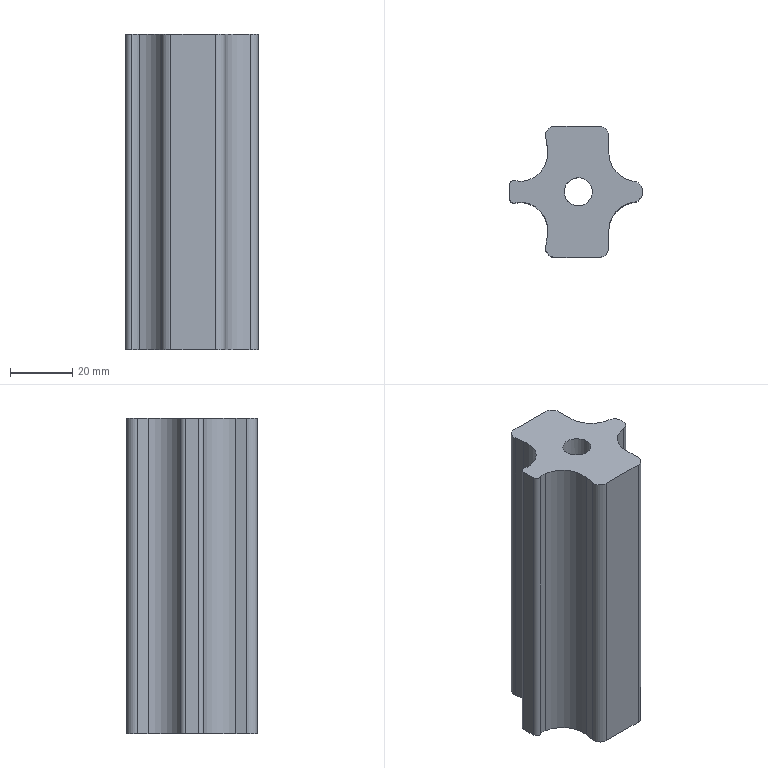Part | STEP file | PN_0031_id862_x_t | 1 solid | 27 faces | box 42.5 x 42 x 101 mm | volume 91343 mm3 | cylinder 16 | plane 11 | commonest cylinder face diameters 6 x6 18.5 x4 3 x2 10 x2 9 x1 14 x1
STEP:
#1=CARTESIAN_POINT('',(343.5,-0.3422,-6.));
#2=VERTEX_POINT('',#1);
#3=CARTESIAN_POINT('',(340.867,-3.32,-6.));
#4=VERTEX_POINT('',#3);
#5=CARTESIAN_POINT('',(340.5,-0.3422,-6.));
#6=DIRECTION('',(0.,0.,-1.));
#7=DIRECTION('',(1.,0.,0.));
#8=AXIS2_PLACEMENT_3D('',#5,#6,#7);
#9=CIRCLE('',#8,3.);
#10=EDGE_CURVE('',#2,#4,#9,.T.);
#11=ORIENTED_EDGE('',*,*,#10,.F.);
#12=CARTESIAN_POINT('',(343.5,-0.3422,95.));
#13=VERTEX_POINT('',#12);
#14=CARTESIAN_POINT('',(343.5,-0.3422,11.));
#15=DIRECTION('',(0.,0.,-1.));
#16=VECTOR('',#15,1.);
#17=LINE('',#14,#16);
#18=EDGE_CURVE('',#13,#2,#17,.T.);
#19=ORIENTED_EDGE('',*,*,#18,.F.);
#20=CARTESIAN_POINT('',(340.867,-3.32,95.));
#21=VERTEX_POINT('',#20);
#22=CARTESIAN_POINT('',(340.5,-0.3422,95.));
#23=DIRECTION('',(0.,0.,-1.));
#24=DIRECTION('',(-1.,0.,0.));
#25=AXIS2_PLACEMENT_3D('',#22,#23,#24);
#26=CIRCLE('',#25,3.);
#27=EDGE_CURVE('',#13,#21,#26,.T.);
#28=ORIENTED_EDGE('',*,*,#27,.T.);
#29=CARTESIAN_POINT('',(340.867,-3.32,11.));
#30=DIRECTION('',(0.,0.,-1.));
#31=VECTOR('',#30,1.);
#32=LINE('',#29,#31);
#33=EDGE_CURVE('',#21,#4,#32,.T.);
#34=ORIENTED_EDGE('',*,*,#33,.T.);
#35=EDGE_LOOP('',(#11,#19,#28,#34));
#36=FACE_OUTER_BOUND('',#35,.T.);
#37=CARTESIAN_POINT('',(340.5,-0.3422,11.));
#38=DIRECTION('',(0.,0.,-1.));
#39=DIRECTION('',(-1.,0.,0.));
#40=AXIS2_PLACEMENT_3D('',#37,#38,#39);
#41=CYLINDRICAL_SURFACE('',#40,3.);
#42=ADVANCED_FACE('',(#36),#41,.T.);
#43=ORIENTED_EDGE('',*,*,#33,.F.);
#44=CARTESIAN_POINT('',(332.75,-12.5,95.));
#45=VERTEX_POINT('',#44);
#46=CARTESIAN_POINT('',(342.,-12.5,95.));
#47=DIRECTION('',(0.,0.,1.));
#48=DIRECTION('',(-1.,0.,0.));
#49=AXIS2_PLACEMENT_3D('',#46,#47,#48);
#50=CIRCLE('',#49,9.25);
#51=EDGE_CURVE('',#21,#45,#50,.T.);
#52=ORIENTED_EDGE('',*,*,#51,.T.);
#53=CARTESIAN_POINT('',(332.75,-12.5,-6.));
#54=VERTEX_POINT('',#53);
#55=CARTESIAN_POINT('',(332.75,-12.5,11.));
#56=DIRECTION('',(0.,0.,-1.));
#57=VECTOR('',#56,1.);
#58=LINE('',#55,#57);
#59=EDGE_CURVE('',#45,#54,#58,.T.);
#60=ORIENTED_EDGE('',*,*,#59,.T.);
#61=CARTESIAN_POINT('',(342.,-12.5,-6.));
#62=DIRECTION('',(0.,0.,1.));
#63=DIRECTION('',(1.,0.,0.));
#64=AXIS2_PLACEMENT_3D('',#61,#62,#63);
#65=CIRCLE('',#64,9.25);
#66=EDGE_CURVE('',#4,#54,#65,.T.);
#67=ORIENTED_EDGE('',*,*,#66,.F.);
#68=EDGE_LOOP('',(#43,#52,#60,#67));
#69=FACE_OUTER_BOUND('',#68,.T.);
#70=CARTESIAN_POINT('',(342.,-12.5,11.));
#71=DIRECTION('',(0.,0.,-1.));
#72=DIRECTION('',(-1.,0.,0.));
#73=AXIS2_PLACEMENT_3D('',#70,#71,#72);
#74=CYLINDRICAL_SURFACE('',#73,9.25);
#75=ADVANCED_FACE('',(#69),#74,.F.);
#76=CARTESIAN_POINT('',(332.75,-18.,95.));
#77=VERTEX_POINT('',#76);
#78=CARTESIAN_POINT('',(332.75,24.687,95.));
#79=DIRECTION('',(0.,-1.,0.));
#80=VECTOR('',#79,1.);
#81=LINE('',#78,#80);
#82=EDGE_CURVE('',#45,#77,#81,.T.);
#83=ORIENTED_EDGE('',*,*,#82,.T.);
#84=CARTESIAN_POINT('',(332.75,-18.,-6.));
#85=VERTEX_POINT('',#84);
#86=CARTESIAN_POINT('',(332.75,-18.,11.));
#87=DIRECTION('',(0.,0.,-1.));
#88=VECTOR('',#87,1.);
#89=LINE('',#86,#88);
#90=EDGE_CURVE('',#77,#85,#89,.T.);
#91=ORIENTED_EDGE('',*,*,#90,.T.);
#92=CARTESIAN_POINT('',(332.75,-96.152,-6.));
#93=DIRECTION('',(0.,-1.,0.));
#94=VECTOR('',#93,1.);
#95=LINE('',#92,#94);
#96=EDGE_CURVE('',#54,#85,#95,.T.);
#97=ORIENTED_EDGE('',*,*,#96,.F.);
#98=ORIENTED_EDGE('',*,*,#59,.F.);
#99=EDGE_LOOP('',(#83,#91,#97,#98));
#100=FACE_OUTER_BOUND('',#99,.T.);
#101=CARTESIAN_POINT('',(332.75,-71.15,11.));
#102=DIRECTION('',(-1.,0.,0.));
#103=DIRECTION('',(0.,1.,0.));
#104=AXIS2_PLACEMENT_3D('',#101,#102,#103);
#105=PLANE('',#104);
#106=ADVANCED_FACE('',(#100),#105,.F.);
#107=CARTESIAN_POINT('',(329.75,-21.,-6.));
#108=VERTEX_POINT('',#107);
#109=CARTESIAN_POINT('',(315.473,-21.,-6.));
#110=VERTEX_POINT('',#109);
#111=CARTESIAN_POINT('',(-201.609,-21.,-6.));
#112=DIRECTION('',(-1.,0.,0.));
#113=VECTOR('',#112,1.);
#114=LINE('',#111,#113);
#115=EDGE_CURVE('',#108,#110,#114,.T.);
#116=ORIENTED_EDGE('',*,*,#115,.F.);
#117=CARTESIAN_POINT('',(329.75,-21.,95.));
#118=VERTEX_POINT('',#117);
#119=CARTESIAN_POINT('',(329.75,-21.,11.));
#120=DIRECTION('',(0.,0.,1.));
#121=VECTOR('',#120,1.);
#122=LINE('',#119,#121);
#123=EDGE_CURVE('',#108,#118,#122,.T.);
#124=ORIENTED_EDGE('',*,*,#123,.T.);
#125=CARTESIAN_POINT('',(315.473,-21.,95.));
#126=VERTEX_POINT('',#125);
#127=CARTESIAN_POINT('',(-114.973,-21.,95.));
#128=DIRECTION('',(-1.,0.,0.));
#129=VECTOR('',#128,1.);
#130=LINE('',#127,#129);
#131=EDGE_CURVE('',#118,#126,#130,.T.);
#132=ORIENTED_EDGE('',*,*,#131,.T.);
#133=CARTESIAN_POINT('',(315.473,-21.,11.));
#134=DIRECTION('',(0.,0.,-1.));
#135=VECTOR('',#134,1.);
#136=LINE('',#133,#135);
#137=EDGE_CURVE('',#126,#110,#136,.T.);
#138=ORIENTED_EDGE('',*,*,#137,.T.);
#139=EDGE_LOOP('',(#116,#124,#132,#138));
#140=FACE_OUTER_BOUND('',#139,.T.);
#141=CARTESIAN_POINT('',(546.19,-21.,11.));
#142=DIRECTION('',(0.,-1.,0.));
#143=DIRECTION('',(-1.,0.,0.));
#144=AXIS2_PLACEMENT_3D('',#141,#142,#143);
#145=PLANE('',#144);
#146=ADVANCED_FACE('',(#140),#145,.T.);
#147=CARTESIAN_POINT('',(312.518,-17.482,-6.));
#148=VERTEX_POINT('',#147);
#149=CARTESIAN_POINT('',(313.111,-14.097,-6.));
#150=VERTEX_POINT('',#149);
#151=CARTESIAN_POINT('',(283.807,-181.252,-6.));
#152=DIRECTION('',(0.1727,0.985,0.));
#153=VECTOR('',#152,1.);
#154=LINE('',#151,#153);
#155=EDGE_CURVE('',#148,#150,#154,.T.);
#156=ORIENTED_EDGE('',*,*,#155,.F.);
#157=CARTESIAN_POINT('',(312.518,-17.482,95.));
#158=VERTEX_POINT('',#157);
#159=CARTESIAN_POINT('',(312.518,-17.482,11.));
#160=DIRECTION('',(0.,0.,1.));
#161=VECTOR('',#160,1.);
#162=LINE('',#159,#161);
#163=EDGE_CURVE('',#148,#158,#162,.T.);
#164=ORIENTED_EDGE('',*,*,#163,.T.);
#165=CARTESIAN_POINT('',(313.111,-14.097,95.));
#166=VERTEX_POINT('',#165);
#167=CARTESIAN_POINT('',(306.943,-49.28,95.));
#168=DIRECTION('',(0.1727,0.985,0.));
#169=VECTOR('',#168,1.);
#170=LINE('',#167,#169);
#171=EDGE_CURVE('',#158,#166,#170,.T.);
#172=ORIENTED_EDGE('',*,*,#171,.T.);
#173=CARTESIAN_POINT('',(313.111,-14.097,11.));
#174=DIRECTION('',(0.,0.,-1.));
#175=VECTOR('',#174,1.);
#176=LINE('',#173,#175);
#177=EDGE_CURVE('',#166,#150,#176,.T.);
#178=ORIENTED_EDGE('',*,*,#177,.T.);
#179=EDGE_LOOP('',(#156,#164,#172,#178));
#180=FACE_OUTER_BOUND('',#179,.T.);
#181=CARTESIAN_POINT('',(313.111,-14.097,11.));
#182=DIRECTION('',(0.985,-0.1727,0.));
#183=DIRECTION('',(-0.1727,-0.985,0.));
#184=AXIS2_PLACEMENT_3D('',#181,#182,#183);
#185=PLANE('',#184);
#186=ADVANCED_FACE('',(#180),#185,.F.);
#187=CARTESIAN_POINT('',(305.382,-3.354,95.));
#188=VERTEX_POINT('',#187);
#189=CARTESIAN_POINT('',(304.,-12.5,95.));
#190=DIRECTION('',(0.,0.,1.));
#191=DIRECTION('',(-1.,0.,0.));
#192=AXIS2_PLACEMENT_3D('',#189,#190,#191);
#193=CIRCLE('',#192,9.25);
#194=EDGE_CURVE('',#166,#188,#193,.T.);
#195=ORIENTED_EDGE('',*,*,#194,.T.);
#196=CARTESIAN_POINT('',(305.382,-3.354,-6.));
#197=VERTEX_POINT('',#196);
#198=CARTESIAN_POINT('',(305.382,-3.354,49.5));
#199=DIRECTION('',(0.,0.,1.));
#200=VECTOR('',#199,1.);
#201=LINE('',#198,#200);
#202=EDGE_CURVE('',#197,#188,#201,.T.);
#203=ORIENTED_EDGE('',*,*,#202,.F.);
#204=CARTESIAN_POINT('',(304.,-12.5,-6.));
#205=DIRECTION('',(0.,0.,1.));
#206=DIRECTION('',(1.,0.,0.));
#207=AXIS2_PLACEMENT_3D('',#204,#205,#206);
#208=CIRCLE('',#207,9.25);
#209=EDGE_CURVE('',#150,#197,#208,.T.);
#210=ORIENTED_EDGE('',*,*,#209,.F.);
#211=ORIENTED_EDGE('',*,*,#177,.F.);
#212=EDGE_LOOP('',(#195,#203,#210,#211));
#213=FACE_OUTER_BOUND('',#212,.T.);
#214=CARTESIAN_POINT('',(304.,-12.5,11.));
#215=DIRECTION('',(0.,0.,-1.));
#216=DIRECTION('',(-1.,0.,0.));
#217=AXIS2_PLACEMENT_3D('',#214,#215,#216);
#218=CYLINDRICAL_SURFACE('',#217,9.25);
#219=ADVANCED_FACE('',(#213),#218,.F.);
#220=CARTESIAN_POINT('',(313.111,14.097,95.));
#221=VERTEX_POINT('',#220);
#222=CARTESIAN_POINT('',(313.111,14.097,-6.));
#223=VERTEX_POINT('',#222);
#224=CARTESIAN_POINT('',(313.111,14.097,11.));
#225=DIRECTION('',(0.,0.,-1.));
#226=VECTOR('',#225,1.);
#227=LINE('',#224,#226);
#228=EDGE_CURVE('',#221,#223,#227,.T.);
#229=ORIENTED_EDGE('',*,*,#228,.T.);
#230=CARTESIAN_POINT('',(305.382,3.354,-6.));
#231=VERTEX_POINT('',#230);
#232=CARTESIAN_POINT('',(304.,12.5,-6.));
#233=DIRECTION('',(0.,0.,1.));
#234=DIRECTION('',(1.,0.,0.));
#235=AXIS2_PLACEMENT_3D('',#232,#233,#234);
#236=CIRCLE('',#235,9.25);
#237=EDGE_CURVE('',#231,#223,#236,.T.);
#238=ORIENTED_EDGE('',*,*,#237,.F.);
#239=CARTESIAN_POINT('',(305.382,3.354,95.));
#240=VERTEX_POINT('',#239);
#241=CARTESIAN_POINT('',(305.382,3.354,49.5));
#242=DIRECTION('',(0.,0.,1.));
#243=VECTOR('',#242,1.);
#244=LINE('',#241,#243);
#245=EDGE_CURVE('',#231,#240,#244,.T.);
#246=ORIENTED_EDGE('',*,*,#245,.T.);
#247=CARTESIAN_POINT('',(304.,12.5,95.));
#248=DIRECTION('',(0.,0.,1.));
#249=DIRECTION('',(-1.,0.,0.));
#250=AXIS2_PLACEMENT_3D('',#247,#248,#249);
#251=CIRCLE('',#250,9.25);
#252=EDGE_CURVE('',#240,#221,#251,.T.);
#253=ORIENTED_EDGE('',*,*,#252,.T.);
#254=EDGE_LOOP('',(#229,#238,#246,#253));
#255=FACE_OUTER_BOUND('',#254,.T.);
#256=CARTESIAN_POINT('',(304.,12.5,11.));
#257=DIRECTION('',(0.,0.,-1.));
#258=DIRECTION('',(-1.,0.,0.));
#259=AXIS2_PLACEMENT_3D('',#256,#257,#258);
#260=CYLINDRICAL_SURFACE('',#259,9.25);
#261=ADVANCED_FACE('',(#255),#260,.F.);
#262=CARTESIAN_POINT('',(312.518,17.482,95.));
#263=VERTEX_POINT('',#262);
#264=CARTESIAN_POINT('',(298.545,97.182,95.));
#265=DIRECTION('',(-0.1727,0.985,0.));
#266=VECTOR('',#265,1.);
#267=LINE('',#264,#266);
#268=EDGE_CURVE('',#221,#263,#267,.T.);
#269=ORIENTED_EDGE('',*,*,#268,.T.);
#270=CARTESIAN_POINT('',(312.518,17.482,-6.));
#271=VERTEX_POINT('',#270);
#272=CARTESIAN_POINT('',(312.518,17.482,11.));
#273=DIRECTION('',(0.,0.,-1.));
#274=VECTOR('',#273,1.);
#275=LINE('',#272,#274);
#276=EDGE_CURVE('',#263,#271,#275,.T.);
#277=ORIENTED_EDGE('',*,*,#276,.T.);
#278=CARTESIAN_POINT('',(316.515,-5.319,-6.));
#279=DIRECTION('',(-0.1727,0.985,0.));
#280=VECTOR('',#279,1.);
#281=LINE('',#278,#280);
#282=EDGE_CURVE('',#223,#271,#281,.T.);
#283=ORIENTED_EDGE('',*,*,#282,.F.);
#284=ORIENTED_EDGE('',*,*,#228,.F.);
#285=EDGE_LOOP('',(#269,#277,#283,#284));
#286=FACE_OUTER_BOUND('',#285,.T.);
#287=CARTESIAN_POINT('',(313.111,14.097,11.));
#288=DIRECTION('',(-0.985,-0.1727,0.));
#289=DIRECTION('',(-0.1727,0.985,0.));
#290=AXIS2_PLACEMENT_3D('',#287,#288,#289);
#291=PLANE('',#290);
#292=ADVANCED_FACE('',(#286),#291,.T.);
#293=CARTESIAN_POINT('',(315.473,21.,95.));
#294=VERTEX_POINT('',#293);
#295=CARTESIAN_POINT('',(329.75,21.,95.));
#296=VERTEX_POINT('',#295);
#297=CARTESIAN_POINT('',(-114.973,21.,95.));
#298=DIRECTION('',(1.,0.,0.));
#299=VECTOR('',#298,1.);
#300=LINE('',#297,#299);
#301=EDGE_CURVE('',#294,#296,#300,.T.);
#302=ORIENTED_EDGE('',*,*,#301,.T.);
#303=CARTESIAN_POINT('',(329.75,21.,-6.));
#304=VERTEX_POINT('',#303);
#305=CARTESIAN_POINT('',(329.75,21.,11.));
#306=DIRECTION('',(0.,0.,-1.));
#307=VECTOR('',#306,1.);
#308=LINE('',#305,#307);
#309=EDGE_CURVE('',#296,#304,#308,.T.);
#310=ORIENTED_EDGE('',*,*,#309,.T.);
#311=CARTESIAN_POINT('',(315.473,21.,-6.));
#312=VERTEX_POINT('',#311);
#313=CARTESIAN_POINT('',(-201.609,21.,-6.));
#314=DIRECTION('',(1.,0.,0.));
#315=VECTOR('',#314,1.);
#316=LINE('',#313,#315);
#317=EDGE_CURVE('',#312,#304,#316,.T.);
#318=ORIENTED_EDGE('',*,*,#317,.F.);
#319=CARTESIAN_POINT('',(315.473,21.,11.));
#320=DIRECTION('',(0.,0.,1.));
#321=VECTOR('',#320,1.);
#322=LINE('',#319,#321);
#323=EDGE_CURVE('',#312,#294,#322,.T.);
#324=ORIENTED_EDGE('',*,*,#323,.T.);
#325=EDGE_LOOP('',(#302,#310,#318,#324));
#326=FACE_OUTER_BOUND('',#325,.T.);
#327=CARTESIAN_POINT('',(266.,21.,11.));
#328=DIRECTION('',(0.,1.,0.));
#329=DIRECTION('',(1.,0.,0.));
#330=AXIS2_PLACEMENT_3D('',#327,#328,#329);
#331=PLANE('',#330);
#332=ADVANCED_FACE('',(#326),#331,.T.);
#333=CARTESIAN_POINT('',(332.75,18.,-6.));
#334=VERTEX_POINT('',#333);
#335=CARTESIAN_POINT('',(332.75,12.5,-6.));
#336=VERTEX_POINT('',#335);
#337=CARTESIAN_POINT('',(332.75,-96.152,-6.));
#338=DIRECTION('',(0.,-1.,0.));
#339=VECTOR('',#338,1.);
#340=LINE('',#337,#339);
#341=EDGE_CURVE('',#334,#336,#340,.T.);
#342=ORIENTED_EDGE('',*,*,#341,.F.);
#343=CARTESIAN_POINT('',(332.75,18.,95.));
#344=VERTEX_POINT('',#343);
#345=CARTESIAN_POINT('',(332.75,18.,11.));
#346=DIRECTION('',(0.,0.,1.));
#347=VECTOR('',#346,1.);
#348=LINE('',#345,#347);
#349=EDGE_CURVE('',#334,#344,#348,.T.);
#350=ORIENTED_EDGE('',*,*,#349,.T.);
#351=CARTESIAN_POINT('',(332.75,12.5,95.));
#352=VERTEX_POINT('',#351);
#353=CARTESIAN_POINT('',(332.75,24.687,95.));
#354=DIRECTION('',(0.,-1.,0.));
#355=VECTOR('',#354,1.);
#356=LINE('',#353,#355);
#357=EDGE_CURVE('',#344,#352,#356,.T.);
#358=ORIENTED_EDGE('',*,*,#357,.T.);
#359=CARTESIAN_POINT('',(332.75,12.5,11.));
#360=DIRECTION('',(0.,0.,-1.));
#361=VECTOR('',#360,1.);
#362=LINE('',#359,#361);
#363=EDGE_CURVE('',#352,#336,#362,.T.);
#364=ORIENTED_EDGE('',*,*,#363,.T.);
#365=EDGE_LOOP('',(#342,#350,#358,#364));
#366=FACE_OUTER_BOUND('',#365,.T.);
#367=CARTESIAN_POINT('',(332.75,71.15,11.));
#368=DIRECTION('',(1.,0.,0.));
#369=DIRECTION('',(0.,-1.,0.));
#370=AXIS2_PLACEMENT_3D('',#367,#368,#369);
#371=PLANE('',#370);
#372=ADVANCED_FACE('',(#366),#371,.T.);
#373=ORIENTED_EDGE('',*,*,#363,.F.);
#374=CARTESIAN_POINT('',(340.867,3.32,95.));
#375=VERTEX_POINT('',#374);
#376=CARTESIAN_POINT('',(342.,12.5,95.));
#377=DIRECTION('',(0.,0.,1.));
#378=DIRECTION('',(-1.,0.,0.));
#379=AXIS2_PLACEMENT_3D('',#376,#377,#378);
#380=CIRCLE('',#379,9.25);
#381=EDGE_CURVE('',#352,#375,#380,.T.);
#382=ORIENTED_EDGE('',*,*,#381,.T.);
#383=CARTESIAN_POINT('',(340.867,3.32,-6.));
#384=VERTEX_POINT('',#383);
#385=CARTESIAN_POINT('',(340.867,3.32,11.));
#386=DIRECTION('',(0.,0.,-1.));
#387=VECTOR('',#386,1.);
#388=LINE('',#385,#387);
#389=EDGE_CURVE('',#375,#384,#388,.T.);
#390=ORIENTED_EDGE('',*,*,#389,.T.);
#391=CARTESIAN_POINT('',(342.,12.5,-6.));
#392=DIRECTION('',(0.,0.,1.));
#393=DIRECTION('',(1.,0.,0.));
#394=AXIS2_PLACEMENT_3D('',#391,#392,#393);
#395=CIRCLE('',#394,9.25);
#396=EDGE_CURVE('',#336,#384,#395,.T.);
#397=ORIENTED_EDGE('',*,*,#396,.F.);
#398=EDGE_LOOP('',(#373,#382,#390,#397));
#399=FACE_OUTER_BOUND('',#398,.T.);
#400=CARTESIAN_POINT('',(342.,12.5,11.));
#401=DIRECTION('',(0.,0.,-1.));
#402=DIRECTION('',(-1.,0.,0.));
#403=AXIS2_PLACEMENT_3D('',#400,#401,#402);
#404=CYLINDRICAL_SURFACE('',#403,9.25);
#405=ADVANCED_FACE('',(#399),#404,.F.);
#406=CARTESIAN_POINT('',(343.5,0.3422,95.));
#407=VERTEX_POINT('',#406);
#408=CARTESIAN_POINT('',(340.5,0.3422,95.));
#409=DIRECTION('',(0.,0.,-1.));
#410=DIRECTION('',(-1.,0.,0.));
#411=AXIS2_PLACEMENT_3D('',#408,#409,#410);
#412=CIRCLE('',#411,3.);
#413=EDGE_CURVE('',#375,#407,#412,.T.);
#414=ORIENTED_EDGE('',*,*,#413,.T.);
#415=CARTESIAN_POINT('',(343.5,0.3422,-6.));
#416=VERTEX_POINT('',#415);
#417=CARTESIAN_POINT('',(343.5,0.3422,11.));
#418=DIRECTION('',(0.,0.,-1.));
#419=VECTOR('',#418,1.);
#420=LINE('',#417,#419);
#421=EDGE_CURVE('',#407,#416,#420,.T.);
#422=ORIENTED_EDGE('',*,*,#421,.T.);
#423=CARTESIAN_POINT('',(340.5,0.3422,-6.));
#424=DIRECTION('',(0.,0.,-1.));
#425=DIRECTION('',(1.,0.,0.));
#426=AXIS2_PLACEMENT_3D('',#423,#424,#425);
#427=CIRCLE('',#426,3.);
#428=EDGE_CURVE('',#384,#416,#427,.T.);
#429=ORIENTED_EDGE('',*,*,#428,.F.);
#430=ORIENTED_EDGE('',*,*,#389,.F.);
#431=EDGE_LOOP('',(#414,#422,#429,#430));
#432=FACE_OUTER_BOUND('',#431,.T.);
#433=CARTESIAN_POINT('',(340.5,0.3422,11.));
#434=DIRECTION('',(0.,0.,-1.));
#435=DIRECTION('',(-1.,0.,0.));
#436=AXIS2_PLACEMENT_3D('',#433,#434,#435);
#437=CYLINDRICAL_SURFACE('',#436,3.);
#438=ADVANCED_FACE('',(#432),#437,.T.);
#439=CARTESIAN_POINT('',(330.,0.,-6.));
#440=VERTEX_POINT('',#439);
#441=CARTESIAN_POINT('',(323.,0.,-6.));
#442=DIRECTION('',(0.,0.,1.));
#443=DIRECTION('',(1.,0.,0.));
#444=AXIS2_PLACEMENT_3D('',#441,#442,#443);
#445=CIRCLE('',#444,7.);
#446=EDGE_CURVE('',#440,#440,#445,.T.);
#447=ORIENTED_EDGE('',*,*,#446,.T.);
#448=EDGE_LOOP('',(#447));
#449=FACE_BOUND('',#448,.T.);
#450=ORIENTED_EDGE('',*,*,#96,.T.);
#451=CARTESIAN_POINT('',(329.75,-18.,-6.));
#452=DIRECTION('',(0.,0.,-1.));
#453=DIRECTION('',(1.,0.,0.));
#454=AXIS2_PLACEMENT_3D('',#451,#452,#453);
#455=CIRCLE('',#454,3.);
#456=EDGE_CURVE('',#85,#108,#455,.T.);
#457=ORIENTED_EDGE('',*,*,#456,.T.);
#458=ORIENTED_EDGE('',*,*,#115,.T.);
#459=CARTESIAN_POINT('',(315.473,-18.,-6.));
#460=DIRECTION('',(0.,0.,-1.));
#461=DIRECTION('',(1.,0.,0.));
#462=AXIS2_PLACEMENT_3D('',#459,#460,#461);
#463=CIRCLE('',#462,3.);
#464=EDGE_CURVE('',#110,#148,#463,.T.);
#465=ORIENTED_EDGE('',*,*,#464,.T.);
#466=ORIENTED_EDGE('',*,*,#155,.T.);
#467=ORIENTED_EDGE('',*,*,#209,.T.);
#468=CARTESIAN_POINT('',(302.993,-3.575,-6.));
#469=VERTEX_POINT('',#468);
#470=CARTESIAN_POINT('',(304.635,-8.298,-6.));
#471=DIRECTION('',(0.,0.,1.));
#472=DIRECTION('',(1.,0.,0.));
#473=AXIS2_PLACEMENT_3D('',#470,#471,#472);
#474=CIRCLE('',#473,5.);
#475=EDGE_CURVE('',#197,#469,#474,.T.);
#476=ORIENTED_EDGE('',*,*,#475,.T.);
#477=CARTESIAN_POINT('',(301.,-2.158,-6.));
#478=VERTEX_POINT('',#477);
#479=CARTESIAN_POINT('',(302.5,-2.158,-6.));
#480=DIRECTION('',(0.,0.,-1.));
#481=DIRECTION('',(1.,0.,0.));
#482=AXIS2_PLACEMENT_3D('',#479,#480,#481);
#483=CIRCLE('',#482,1.5);
#484=EDGE_CURVE('',#469,#478,#483,.T.);
#485=ORIENTED_EDGE('',*,*,#484,.T.);
#486=CARTESIAN_POINT('',(301.,2.158,-6.));
#487=VERTEX_POINT('',#486);
#488=CARTESIAN_POINT('',(301.,-96.152,-6.));
#489=DIRECTION('',(0.,1.,0.));
#490=VECTOR('',#489,1.);
#491=LINE('',#488,#490);
#492=EDGE_CURVE('',#478,#487,#491,.T.);
#493=ORIENTED_EDGE('',*,*,#492,.T.);
#494=CARTESIAN_POINT('',(302.993,3.575,-6.));
#495=VERTEX_POINT('',#494);
#496=CARTESIAN_POINT('',(302.5,2.158,-6.));
#497=DIRECTION('',(0.,0.,-1.));
#498=DIRECTION('',(1.,0.,0.));
#499=AXIS2_PLACEMENT_3D('',#496,#497,#498);
#500=CIRCLE('',#499,1.5);
#501=EDGE_CURVE('',#487,#495,#500,.T.);
#502=ORIENTED_EDGE('',*,*,#501,.T.);
#503=CARTESIAN_POINT('',(304.635,8.298,-6.));
#504=DIRECTION('',(0.,0.,1.));
#505=DIRECTION('',(1.,0.,0.));
#506=AXIS2_PLACEMENT_3D('',#503,#504,#505);
#507=CIRCLE('',#506,5.);
#508=EDGE_CURVE('',#495,#231,#507,.T.);
#509=ORIENTED_EDGE('',*,*,#508,.T.);
#510=ORIENTED_EDGE('',*,*,#237,.T.);
#511=ORIENTED_EDGE('',*,*,#282,.T.);
#512=CARTESIAN_POINT('',(315.473,18.,-6.));
#513=DIRECTION('',(0.,0.,-1.));
#514=DIRECTION('',(1.,0.,0.));
#515=AXIS2_PLACEMENT_3D('',#512,#513,#514);
#516=CIRCLE('',#515,3.);
#517=EDGE_CURVE('',#271,#312,#516,.T.);
#518=ORIENTED_EDGE('',*,*,#517,.T.);
#519=ORIENTED_EDGE('',*,*,#317,.T.);
#520=CARTESIAN_POINT('',(329.75,18.,-6.));
#521=DIRECTION('',(0.,0.,-1.));
#522=DIRECTION('',(1.,0.,0.));
#523=AXIS2_PLACEMENT_3D('',#520,#521,#522);
#524=CIRCLE('',#523,3.);
#525=EDGE_CURVE('',#304,#334,#524,.T.);
#526=ORIENTED_EDGE('',*,*,#525,.T.);
#527=ORIENTED_EDGE('',*,*,#341,.T.);
#528=ORIENTED_EDGE('',*,*,#396,.T.);
#529=ORIENTED_EDGE('',*,*,#428,.T.);
#530=CARTESIAN_POINT('',(343.5,-96.152,-6.));
#531=DIRECTION('',(0.,-1.,0.));
#532=VECTOR('',#531,1.);
#533=LINE('',#530,#532);
#534=EDGE_CURVE('',#416,#2,#533,.T.);
#535=ORIENTED_EDGE('',*,*,#534,.T.);
#536=ORIENTED_EDGE('',*,*,#10,.T.);
#537=ORIENTED_EDGE('',*,*,#66,.T.);
#538=EDGE_LOOP('',(#450,#457,#458,#465,#466,#467,#476,#485,#493,#502,#509,#510,#511,#518,#519,#526,#527,#528,#529,#535,#536,#537));
#539=FACE_BOUND('',#538,.T.);
#540=CARTESIAN_POINT('',(-201.609,-96.152,-6.));
#541=DIRECTION('',(0.,0.,1.));
#542=DIRECTION('',(1.,0.,0.));
#543=AXIS2_PLACEMENT_3D('',#540,#541,#542);
#544=PLANE('',#543);
#545=ADVANCED_FACE('',(#449,#539),#544,.F.);
#546=CARTESIAN_POINT('',(318.5,0.,95.));
#547=VERTEX_POINT('',#546);
#548=CARTESIAN_POINT('',(323.,0.,95.));
#549=DIRECTION('',(0.,0.,-1.));
#550=DIRECTION('',(-1.,0.,0.));
#551=AXIS2_PLACEMENT_3D('',#548,#549,#550);
#552=CIRCLE('',#551,4.5);
#553=EDGE_CURVE('',#547,#547,#552,.T.);
#554=ORIENTED_EDGE('',*,*,#553,.T.);
#555=EDGE_LOOP('',(#554));
#556=FACE_BOUND('',#555,.T.);
#557=ORIENTED_EDGE('',*,*,#131,.F.);
#558=CARTESIAN_POINT('',(329.75,-18.,95.));
#559=DIRECTION('',(0.,0.,1.));
#560=DIRECTION('',(-1.,0.,0.));
#561=AXIS2_PLACEMENT_3D('',#558,#559,#560);
#562=CIRCLE('',#561,3.);
#563=EDGE_CURVE('',#118,#77,#562,.T.);
#564=ORIENTED_EDGE('',*,*,#563,.T.);
#565=ORIENTED_EDGE('',*,*,#82,.F.);
#566=ORIENTED_EDGE('',*,*,#51,.F.);
#567=ORIENTED_EDGE('',*,*,#27,.F.);
#568=CARTESIAN_POINT('',(343.5,24.687,95.));
#569=DIRECTION('',(0.,-1.,0.));
#570=VECTOR('',#569,1.);
#571=LINE('',#568,#570);
#572=EDGE_CURVE('',#407,#13,#571,.T.);
#573=ORIENTED_EDGE('',*,*,#572,.F.);
#574=ORIENTED_EDGE('',*,*,#413,.F.);
#575=ORIENTED_EDGE('',*,*,#381,.F.);
#576=ORIENTED_EDGE('',*,*,#357,.F.);
#577=CARTESIAN_POINT('',(329.75,18.,95.));
#578=DIRECTION('',(0.,0.,1.));
#579=DIRECTION('',(-1.,0.,0.));
#580=AXIS2_PLACEMENT_3D('',#577,#578,#579);
#581=CIRCLE('',#580,3.);
#582=EDGE_CURVE('',#344,#296,#581,.T.);
#583=ORIENTED_EDGE('',*,*,#582,.T.);
#584=ORIENTED_EDGE('',*,*,#301,.F.);
#585=CARTESIAN_POINT('',(315.473,18.,95.));
#586=DIRECTION('',(0.,0.,1.));
#587=DIRECTION('',(-1.,0.,0.));
#588=AXIS2_PLACEMENT_3D('',#585,#586,#587);
#589=CIRCLE('',#588,3.);
#590=EDGE_CURVE('',#294,#263,#589,.T.);
#591=ORIENTED_EDGE('',*,*,#590,.T.);
#592=ORIENTED_EDGE('',*,*,#268,.F.);
#593=ORIENTED_EDGE('',*,*,#252,.F.);
#594=CARTESIAN_POINT('',(302.993,3.575,95.));
#595=VERTEX_POINT('',#594);
#596=CARTESIAN_POINT('',(304.635,8.298,95.));
#597=DIRECTION('',(0.,0.,1.));
#598=DIRECTION('',(-1.,0.,0.));
#599=AXIS2_PLACEMENT_3D('',#596,#597,#598);
#600=CIRCLE('',#599,5.);
#601=EDGE_CURVE('',#595,#240,#600,.T.);
#602=ORIENTED_EDGE('',*,*,#601,.F.);
#603=CARTESIAN_POINT('',(301.,2.158,95.));
#604=VERTEX_POINT('',#603);
#605=CARTESIAN_POINT('',(302.5,2.158,95.));
#606=DIRECTION('',(0.,0.,-1.));
#607=DIRECTION('',(-1.,0.,0.));
#608=AXIS2_PLACEMENT_3D('',#605,#606,#607);
#609=CIRCLE('',#608,1.5);
#610=EDGE_CURVE('',#604,#595,#609,.T.);
#611=ORIENTED_EDGE('',*,*,#610,.F.);
#612=CARTESIAN_POINT('',(301.,-2.158,95.));
#613=VERTEX_POINT('',#612);
#614=CARTESIAN_POINT('',(301.,24.687,95.));
#615=DIRECTION('',(0.,1.,0.));
#616=VECTOR('',#615,1.);
#617=LINE('',#614,#616);
#618=EDGE_CURVE('',#613,#604,#617,.T.);
#619=ORIENTED_EDGE('',*,*,#618,.F.);
#620=CARTESIAN_POINT('',(302.993,-3.575,95.));
#621=VERTEX_POINT('',#620);
#622=CARTESIAN_POINT('',(302.5,-2.158,95.));
#623=DIRECTION('',(0.,0.,-1.));
#624=DIRECTION('',(-1.,0.,0.));
#625=AXIS2_PLACEMENT_3D('',#622,#623,#624);
#626=CIRCLE('',#625,1.5);
#627=EDGE_CURVE('',#621,#613,#626,.T.);
#628=ORIENTED_EDGE('',*,*,#627,.F.);
#629=CARTESIAN_POINT('',(304.635,-8.298,95.));
#630=DIRECTION('',(0.,0.,1.));
#631=DIRECTION('',(-1.,0.,0.));
#632=AXIS2_PLACEMENT_3D('',#629,#630,#631);
#633=CIRCLE('',#632,5.);
#634=EDGE_CURVE('',#188,#621,#633,.T.);
#635=ORIENTED_EDGE('',*,*,#634,.F.);
#636=ORIENTED_EDGE('',*,*,#194,.F.);
#637=ORIENTED_EDGE('',*,*,#171,.F.);
#638=CARTESIAN_POINT('',(315.473,-18.,95.));
#639=DIRECTION('',(0.,0.,1.));
#640=DIRECTION('',(-1.,0.,0.));
#641=AXIS2_PLACEMENT_3D('',#638,#639,#640);
#642=CIRCLE('',#641,3.);
#643=EDGE_CURVE('',#158,#126,#642,.T.);
#644=ORIENTED_EDGE('',*,*,#643,.T.);
#645=EDGE_LOOP('',(#557,#564,#565,#566,#567,#573,#574,#575,#576,#583,#584,#591,#592,#593,#602,#611,#619,#628,#635,#636,#637,#644));
#646=FACE_BOUND('',#645,.T.);
#647=CARTESIAN_POINT('',(-114.973,24.687,95.));
#648=DIRECTION('',(0.,0.,-1.));
#649=DIRECTION('',(-1.,0.,0.));
#650=AXIS2_PLACEMENT_3D('',#647,#648,#649);
#651=PLANE('',#650);
#652=ADVANCED_FACE('',(#556,#646),#651,.F.);
#653=ORIENTED_EDGE('',*,*,#484,.F.);
#654=CARTESIAN_POINT('',(302.993,-3.575,11.));
#655=DIRECTION('',(0.,0.,-1.));
#656=VECTOR('',#655,1.);
#657=LINE('',#654,#656);
#658=EDGE_CURVE('',#621,#469,#657,.T.);
#659=ORIENTED_EDGE('',*,*,#658,.F.);
#660=ORIENTED_EDGE('',*,*,#627,.T.);
#661=CARTESIAN_POINT('',(301.,-2.158,11.));
#662=DIRECTION('',(0.,0.,-1.));
#663=VECTOR('',#662,1.);
#664=LINE('',#661,#663);
#665=EDGE_CURVE('',#613,#478,#664,.T.);
#666=ORIENTED_EDGE('',*,*,#665,.T.);
#667=EDGE_LOOP('',(#653,#659,#660,#666));
#668=FACE_OUTER_BOUND('',#667,.T.);
#669=CARTESIAN_POINT('',(302.5,-2.158,11.));
#670=DIRECTION('',(0.,0.,-1.));
#671=DIRECTION('',(-1.,0.,0.));
#672=AXIS2_PLACEMENT_3D('',#669,#670,#671);
#673=CYLINDRICAL_SURFACE('',#672,1.5);
#674=ADVANCED_FACE('',(#668),#673,.T.);
#675=ORIENTED_EDGE('',*,*,#665,.F.);
#676=ORIENTED_EDGE('',*,*,#618,.T.);
#677=CARTESIAN_POINT('',(301.,2.158,11.));
#678=DIRECTION('',(0.,0.,-1.));
#679=VECTOR('',#678,1.);
#680=LINE('',#677,#679);
#681=EDGE_CURVE('',#604,#487,#680,.T.);
#682=ORIENTED_EDGE('',*,*,#681,.T.);
#683=ORIENTED_EDGE('',*,*,#492,.F.);
#684=EDGE_LOOP('',(#675,#676,#682,#683));
#685=FACE_OUTER_BOUND('',#684,.T.);
#686=CARTESIAN_POINT('',(301.,-13.,11.));
#687=DIRECTION('',(-1.,0.,0.));
#688=DIRECTION('',(0.,1.,0.));
#689=AXIS2_PLACEMENT_3D('',#686,#687,#688);
#690=PLANE('',#689);
#691=ADVANCED_FACE('',(#685),#690,.T.);
#692=ORIENTED_EDGE('',*,*,#610,.T.);
#693=CARTESIAN_POINT('',(302.993,3.575,11.));
#694=DIRECTION('',(0.,0.,-1.));
#695=VECTOR('',#694,1.);
#696=LINE('',#693,#695);
#697=EDGE_CURVE('',#595,#495,#696,.T.);
#698=ORIENTED_EDGE('',*,*,#697,.T.);
#699=ORIENTED_EDGE('',*,*,#501,.F.);
#700=ORIENTED_EDGE('',*,*,#681,.F.);
#701=EDGE_LOOP('',(#692,#698,#699,#700));
#702=FACE_OUTER_BOUND('',#701,.T.);
#703=CARTESIAN_POINT('',(302.5,2.158,11.));
#704=DIRECTION('',(0.,0.,-1.));
#705=DIRECTION('',(-1.,0.,0.));
#706=AXIS2_PLACEMENT_3D('',#703,#704,#705);
#707=CYLINDRICAL_SURFACE('',#706,1.5);
#708=ADVANCED_FACE('',(#702),#707,.T.);
#709=ORIENTED_EDGE('',*,*,#697,.F.);
#710=ORIENTED_EDGE('',*,*,#601,.T.);
#711=ORIENTED_EDGE('',*,*,#245,.F.);
#712=ORIENTED_EDGE('',*,*,#508,.F.);
#713=EDGE_LOOP('',(#709,#710,#711,#712));
#714=FACE_OUTER_BOUND('',#713,.T.);
#715=CARTESIAN_POINT('',(304.635,8.298,11.));
#716=DIRECTION('',(0.,0.,-1.));
#717=DIRECTION('',(-1.,0.,0.));
#718=AXIS2_PLACEMENT_3D('',#715,#716,#717);
#719=CYLINDRICAL_SURFACE('',#718,5.);
#720=ADVANCED_FACE('',(#714),#719,.F.);
#721=ORIENTED_EDGE('',*,*,#475,.F.);
#722=ORIENTED_EDGE('',*,*,#202,.T.);
#723=ORIENTED_EDGE('',*,*,#634,.T.);
#724=ORIENTED_EDGE('',*,*,#658,.T.);
#725=EDGE_LOOP('',(#721,#722,#723,#724));
#726=FACE_OUTER_BOUND('',#725,.T.);
#727=CARTESIAN_POINT('',(304.635,-8.298,11.));
#728=DIRECTION('',(0.,0.,-1.));
#729=DIRECTION('',(-1.,0.,0.));
#730=AXIS2_PLACEMENT_3D('',#727,#728,#729);
#731=CYLINDRICAL_SURFACE('',#730,5.);
#732=ADVANCED_FACE('',(#726),#731,.F.);
#733=ORIENTED_EDGE('',*,*,#421,.F.);
#734=ORIENTED_EDGE('',*,*,#572,.T.);
#735=ORIENTED_EDGE('',*,*,#18,.T.);
#736=ORIENTED_EDGE('',*,*,#534,.F.);
#737=EDGE_LOOP('',(#733,#734,#735,#736));
#738=FACE_OUTER_BOUND('',#737,.T.);
#739=CARTESIAN_POINT('',(343.5,52.192,11.));
#740=DIRECTION('',(-1.,0.,0.));
#741=DIRECTION('',(0.,1.,0.));
#742=AXIS2_PLACEMENT_3D('',#739,#740,#741);
#743=PLANE('',#742);
#744=ADVANCED_FACE('',(#738),#743,.F.);
#745=ORIENTED_EDGE('',*,*,#563,.F.);
#746=ORIENTED_EDGE('',*,*,#123,.F.);
#747=ORIENTED_EDGE('',*,*,#456,.F.);
#748=ORIENTED_EDGE('',*,*,#90,.F.);
#749=EDGE_LOOP('',(#745,#746,#747,#748));
#750=FACE_OUTER_BOUND('',#749,.T.);
#751=CARTESIAN_POINT('',(329.75,-18.,11.));
#752=DIRECTION('',(0.,0.,1.));
#753=DIRECTION('',(1.,0.,0.));
#754=AXIS2_PLACEMENT_3D('',#751,#752,#753);
#755=CYLINDRICAL_SURFACE('',#754,3.);
#756=ADVANCED_FACE('',(#750),#755,.T.);
#757=ORIENTED_EDGE('',*,*,#643,.F.);
#758=ORIENTED_EDGE('',*,*,#163,.F.);
#759=ORIENTED_EDGE('',*,*,#464,.F.);
#760=ORIENTED_EDGE('',*,*,#137,.F.);
#761=EDGE_LOOP('',(#757,#758,#759,#760));
#762=FACE_OUTER_BOUND('',#761,.T.);
#763=CARTESIAN_POINT('',(315.473,-18.,11.));
#764=DIRECTION('',(0.,0.,1.));
#765=DIRECTION('',(1.,0.,0.));
#766=AXIS2_PLACEMENT_3D('',#763,#764,#765);
#767=CYLINDRICAL_SURFACE('',#766,3.);
#768=ADVANCED_FACE('',(#762),#767,.T.);
#769=ORIENTED_EDGE('',*,*,#582,.F.);
#770=ORIENTED_EDGE('',*,*,#349,.F.);
#771=ORIENTED_EDGE('',*,*,#525,.F.);
#772=ORIENTED_EDGE('',*,*,#309,.F.);
#773=EDGE_LOOP('',(#769,#770,#771,#772));
#774=FACE_OUTER_BOUND('',#773,.T.);
#775=CARTESIAN_POINT('',(329.75,18.,11.));
#776=DIRECTION('',(0.,0.,-1.));
#777=DIRECTION('',(-1.,0.,0.));
#778=AXIS2_PLACEMENT_3D('',#775,#776,#777);
#779=CYLINDRICAL_SURFACE('',#778,3.);
#780=ADVANCED_FACE('',(#774),#779,.T.);
#781=ORIENTED_EDGE('',*,*,#590,.F.);
#782=ORIENTED_EDGE('',*,*,#323,.F.);
#783=ORIENTED_EDGE('',*,*,#517,.F.);
#784=ORIENTED_EDGE('',*,*,#276,.F.);
#785=EDGE_LOOP('',(#781,#782,#783,#784));
#786=FACE_OUTER_BOUND('',#785,.T.);
#787=CARTESIAN_POINT('',(315.473,18.,11.));
#788=DIRECTION('',(0.,0.,-1.));
#789=DIRECTION('',(-1.,0.,0.));
#790=AXIS2_PLACEMENT_3D('',#787,#788,#789);
#791=CYLINDRICAL_SURFACE('',#790,3.);
#792=ADVANCED_FACE('',(#786),#791,.T.);
#793=CARTESIAN_POINT('',(323.,-4.5,75.));
#794=VERTEX_POINT('',#793);
#795=CARTESIAN_POINT('',(323.,0.,75.));
#796=DIRECTION('',(0.,0.,1.));
#797=DIRECTION('',(0.,-1.,0.));
#798=AXIS2_PLACEMENT_3D('',#795,#796,#797);
#799=CIRCLE('',#798,4.5);
#800=EDGE_CURVE('',#794,#794,#799,.T.);
#801=ORIENTED_EDGE('',*,*,#800,.F.);
#802=EDGE_LOOP('',(#801));
#803=FACE_BOUND('',#802,.T.);
#804=ORIENTED_EDGE('',*,*,#553,.F.);
#805=EDGE_LOOP('',(#804));
#806=FACE_BOUND('',#805,.T.);
#807=CARTESIAN_POINT('',(323.,0.,105.));
#808=DIRECTION('',(0.,0.,-1.));
#809=DIRECTION('',(0.,1.,0.));
#810=AXIS2_PLACEMENT_3D('',#807,#808,#809);
#811=CYLINDRICAL_SURFACE('',#810,4.5);
#812=ADVANCED_FACE('',(#803,#806),#811,.F.);
#813=ORIENTED_EDGE('',*,*,#800,.T.);
#814=EDGE_LOOP('',(#813));
#815=FACE_BOUND('',#814,.T.);
#816=CARTESIAN_POINT('',(323.,7.,75.));
#817=VERTEX_POINT('',#816);
#818=CARTESIAN_POINT('',(323.,0.,75.));
#819=DIRECTION('',(0.,0.,1.));
#820=DIRECTION('',(0.,1.,0.));
#821=AXIS2_PLACEMENT_3D('',#818,#819,#820);
#822=CIRCLE('',#821,7.);
#823=EDGE_CURVE('',#817,#817,#822,.T.);
#824=ORIENTED_EDGE('',*,*,#823,.F.);
#825=EDGE_LOOP('',(#824));
#826=FACE_BOUND('',#825,.T.);
#827=CARTESIAN_POINT('',(323.,0.,75.));
#828=DIRECTION('',(0.,0.,1.));
#829=DIRECTION('',(0.,-1.,0.));
#830=AXIS2_PLACEMENT_3D('',#827,#828,#829);
#831=PLANE('',#830);
#832=ADVANCED_FACE('',(#815,#826),#831,.F.);
#833=ORIENTED_EDGE('',*,*,#446,.F.);
#834=EDGE_LOOP('',(#833));
#835=FACE_BOUND('',#834,.T.);
#836=ORIENTED_EDGE('',*,*,#823,.T.);
#837=EDGE_LOOP('',(#836));
#838=FACE_BOUND('',#837,.T.);
#839=CARTESIAN_POINT('',(323.,0.,75.));
#840=DIRECTION('',(0.,0.,-1.));
#841=DIRECTION('',(0.,1.,0.));
#842=AXIS2_PLACEMENT_3D('',#839,#840,#841);
#843=CYLINDRICAL_SURFACE('',#842,7.);
#844=ADVANCED_FACE('',(#835,#838),#843,.F.);
#845=CLOSED_SHELL('',(#42,#75,#106,#146,#186,#219,#261,#292,#332,#372,#405,#438,#545,#652,#674,#691,#708,#720,#732,#744,#756,#768,#780,#792,#812,#832,#844));
#846=MANIFOLD_SOLID_BREP('',#845);
#847=(LENGTH_UNIT()NAMED_UNIT(*)SI_UNIT(.MILLI.,.METRE.));
#848=UNCERTAINTY_MEASURE_WITH_UNIT(LENGTH_MEASURE(0.00002),#847,'','');
#849=(NAMED_UNIT(*)PLANE_ANGLE_UNIT()SI_UNIT($,.RADIAN.));
#850=PLANE_ANGLE_MEASURE_WITH_UNIT(PLANE_ANGLE_MEASURE(0.01745),#849);
#851=DIMENSIONAL_EXPONENTS(0.,0.,0.,0.,0.,0.,0.);
#852=(CONVERSION_BASED_UNIT('DEGREE',#850)NAMED_UNIT(#851)PLANE_ANGLE_UNIT());
#853=(NAMED_UNIT(*)SI_UNIT($,.STERADIAN.)SOLID_ANGLE_UNIT());
#854=(GEOMETRIC_REPRESENTATION_CONTEXT(3)GLOBAL_UNCERTAINTY_ASSIGNED_CONTEXT((#848))GLOBAL_UNIT_ASSIGNED_CONTEXT((#847,#852,#853))REPRESENTATION_CONTEXT('',''));
#855=ADVANCED_BREP_SHAPE_REPRESENTATION('',(#846),#854);